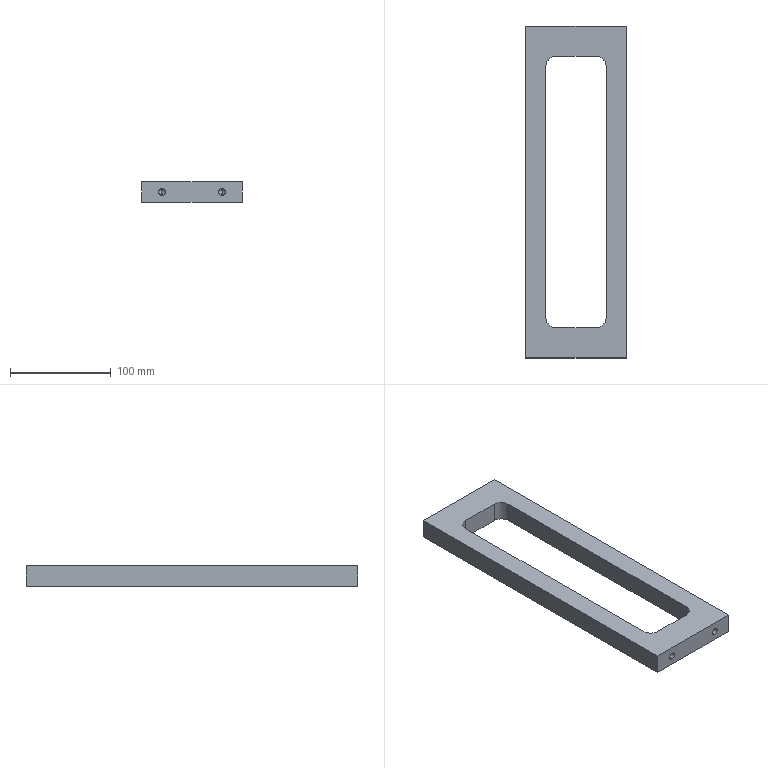Part | SolidWorks | features BaseBody 1 | 1 solid | 22 faces | box 100 x 330 x 20 mm | volume 336233 mm3 | plane 10 | cylinder 8 | cone 4 | commonest cylinder face diameters 6.8 x4 20 x4
STEP:
#1=CARTESIAN_POINT('',(30.,-145.25,3.4));
#2=VERTEX_POINT('',#1);
#3=CARTESIAN_POINT('',(30.,-145.25,-3.4));
#4=VERTEX_POINT('',#3);
#5=CARTESIAN_POINT('',(30.,-145.25,0.));
#6=DIRECTION('',(0.,-1.,0.));
#7=DIRECTION('',(0.,0.,-1.));
#8=AXIS2_PLACEMENT_3D('',#5,#6,#7);
#9=CIRCLE('',#8,3.4);
#10=EDGE_CURVE('',#2,#4,#9,.T.);
#11=ORIENTED_EDGE('',*,*,#10,.F.);
#12=CARTESIAN_POINT('',(30.,-165.,3.4));
#13=VERTEX_POINT('',#12);
#14=CARTESIAN_POINT('',(30.,-165.,3.4));
#15=DIRECTION('',(0.,-1.,0.));
#16=VECTOR('',#15,1000.);
#17=LINE('',#14,#16);
#18=EDGE_CURVE('',#2,#13,#17,.T.);
#19=ORIENTED_EDGE('',*,*,#18,.T.);
#20=CARTESIAN_POINT('',(30.,-165.,-3.4));
#21=VERTEX_POINT('',#20);
#22=CARTESIAN_POINT('',(30.,-165.,0.));
#23=DIRECTION('',(0.,-1.,0.));
#24=DIRECTION('',(0.,0.,-1.));
#25=AXIS2_PLACEMENT_3D('',#22,#23,#24);
#26=CIRCLE('',#25,3.4);
#27=EDGE_CURVE('',#13,#21,#26,.T.);
#28=ORIENTED_EDGE('',*,*,#27,.T.);
#29=CARTESIAN_POINT('',(30.,-165.,-3.4));
#30=DIRECTION('',(0.,-1.,0.));
#31=VECTOR('',#30,1000.);
#32=LINE('',#29,#31);
#33=EDGE_CURVE('',#4,#21,#32,.T.);
#34=ORIENTED_EDGE('',*,*,#33,.F.);
#35=EDGE_LOOP('',(#11,#19,#28,#34));
#36=FACE_OUTER_BOUND('',#35,.T.);
#37=CARTESIAN_POINT('',(30.,-165.,0.));
#38=DIRECTION('',(0.,-1.,0.));
#39=DIRECTION('',(0.,0.,-1.));
#40=AXIS2_PLACEMENT_3D('',#37,#38,#39);
#41=CYLINDRICAL_SURFACE('',#40,3.4);
#42=ADVANCED_FACE('',(#36),#41,.F.);
#43=CARTESIAN_POINT('',(30.,-143.207,0.));
#44=VERTEX_POINT('',#43);
#45=CARTESIAN_POINT('',(30.,-145.25,-3.4));
#46=DIRECTION('',(0.,-0.515,-0.8572));
#47=VECTOR('',#46,1000.);
#48=LINE('',#45,#47);
#49=EDGE_CURVE('',#44,#4,#48,.T.);
#50=ORIENTED_EDGE('',*,*,#49,.F.);
#51=CARTESIAN_POINT('',(30.,-145.25,3.4));
#52=DIRECTION('',(0.,-0.515,0.8572));
#53=VECTOR('',#52,1000.);
#54=LINE('',#51,#53);
#55=EDGE_CURVE('',#44,#2,#54,.T.);
#56=ORIENTED_EDGE('',*,*,#55,.T.);
#57=ORIENTED_EDGE('',*,*,#10,.T.);
#58=EDGE_LOOP('',(#50,#56,#57));
#59=FACE_OUTER_BOUND('',#58,.T.);
#60=CARTESIAN_POINT('',(30.,-145.25,0.));
#61=DIRECTION('',(0.,-1.,0.));
#62=DIRECTION('',(0.,0.,-1.));
#63=AXIS2_PLACEMENT_3D('',#60,#61,#62);
#64=CONICAL_SURFACE('',#63,3.4,1.03);
#65=ADVANCED_FACE('',(#59),#64,.F.);
#66=CARTESIAN_POINT('',(-30.,-145.25,3.4));
#67=VERTEX_POINT('',#66);
#68=CARTESIAN_POINT('',(-30.,-145.25,-3.4));
#69=VERTEX_POINT('',#68);
#70=CARTESIAN_POINT('',(-30.,-145.25,0.));
#71=DIRECTION('',(0.,-1.,0.));
#72=DIRECTION('',(0.,0.,-1.));
#73=AXIS2_PLACEMENT_3D('',#70,#71,#72);
#74=CIRCLE('',#73,3.4);
#75=EDGE_CURVE('',#67,#69,#74,.T.);
#76=ORIENTED_EDGE('',*,*,#75,.F.);
#77=CARTESIAN_POINT('',(-30.,-165.,3.4));
#78=VERTEX_POINT('',#77);
#79=CARTESIAN_POINT('',(-30.,-165.,3.4));
#80=DIRECTION('',(0.,-1.,0.));
#81=VECTOR('',#80,1000.);
#82=LINE('',#79,#81);
#83=EDGE_CURVE('',#67,#78,#82,.T.);
#84=ORIENTED_EDGE('',*,*,#83,.T.);
#85=CARTESIAN_POINT('',(-30.,-165.,-3.4));
#86=VERTEX_POINT('',#85);
#87=CARTESIAN_POINT('',(-30.,-165.,0.));
#88=DIRECTION('',(0.,-1.,0.));
#89=DIRECTION('',(0.,0.,-1.));
#90=AXIS2_PLACEMENT_3D('',#87,#88,#89);
#91=CIRCLE('',#90,3.4);
#92=EDGE_CURVE('',#78,#86,#91,.T.);
#93=ORIENTED_EDGE('',*,*,#92,.T.);
#94=CARTESIAN_POINT('',(-30.,-165.,-3.4));
#95=DIRECTION('',(0.,-1.,0.));
#96=VECTOR('',#95,1000.);
#97=LINE('',#94,#96);
#98=EDGE_CURVE('',#69,#86,#97,.T.);
#99=ORIENTED_EDGE('',*,*,#98,.F.);
#100=EDGE_LOOP('',(#76,#84,#93,#99));
#101=FACE_OUTER_BOUND('',#100,.T.);
#102=CARTESIAN_POINT('',(-30.,-165.,0.));
#103=DIRECTION('',(0.,-1.,0.));
#104=DIRECTION('',(0.,0.,-1.));
#105=AXIS2_PLACEMENT_3D('',#102,#103,#104);
#106=CYLINDRICAL_SURFACE('',#105,3.4);
#107=ADVANCED_FACE('',(#101),#106,.F.);
#108=CARTESIAN_POINT('',(-30.,-143.207,0.));
#109=VERTEX_POINT('',#108);
#110=CARTESIAN_POINT('',(-30.,-145.25,-3.4));
#111=DIRECTION('',(0.,-0.515,-0.8572));
#112=VECTOR('',#111,1000.);
#113=LINE('',#110,#112);
#114=EDGE_CURVE('',#109,#69,#113,.T.);
#115=ORIENTED_EDGE('',*,*,#114,.F.);
#116=CARTESIAN_POINT('',(-30.,-145.25,3.4));
#117=DIRECTION('',(0.,-0.515,0.8572));
#118=VECTOR('',#117,1000.);
#119=LINE('',#116,#118);
#120=EDGE_CURVE('',#109,#67,#119,.T.);
#121=ORIENTED_EDGE('',*,*,#120,.T.);
#122=ORIENTED_EDGE('',*,*,#75,.T.);
#123=EDGE_LOOP('',(#115,#121,#122));
#124=FACE_OUTER_BOUND('',#123,.T.);
#125=CARTESIAN_POINT('',(-30.,-145.25,0.));
#126=DIRECTION('',(0.,-1.,0.));
#127=DIRECTION('',(0.,0.,-1.));
#128=AXIS2_PLACEMENT_3D('',#125,#126,#127);
#129=CONICAL_SURFACE('',#128,3.4,1.03);
#130=ADVANCED_FACE('',(#124),#129,.F.);
#131=CARTESIAN_POINT('',(-50.,165.,-10.));
#132=VERTEX_POINT('',#131);
#133=CARTESIAN_POINT('',(-50.,-165.,-10.));
#134=VERTEX_POINT('',#133);
#135=CARTESIAN_POINT('',(-50.,165.,-10.));
#136=DIRECTION('',(0.,-1.,0.));
#137=VECTOR('',#136,1000.);
#138=LINE('',#135,#137);
#139=EDGE_CURVE('',#132,#134,#138,.T.);
#140=ORIENTED_EDGE('',*,*,#139,.T.);
#141=CARTESIAN_POINT('',(-50.,-165.,10.));
#142=VERTEX_POINT('',#141);
#143=CARTESIAN_POINT('',(-50.,-165.,10.));
#144=DIRECTION('',(0.,0.,-1.));
#145=VECTOR('',#144,1000.);
#146=LINE('',#143,#145);
#147=EDGE_CURVE('',#142,#134,#146,.T.);
#148=ORIENTED_EDGE('',*,*,#147,.F.);
#149=CARTESIAN_POINT('',(-50.,165.,10.));
#150=VERTEX_POINT('',#149);
#151=CARTESIAN_POINT('',(-50.,165.,10.));
#152=DIRECTION('',(0.,-1.,0.));
#153=VECTOR('',#152,1000.);
#154=LINE('',#151,#153);
#155=EDGE_CURVE('',#150,#142,#154,.T.);
#156=ORIENTED_EDGE('',*,*,#155,.F.);
#157=CARTESIAN_POINT('',(-50.,165.,10.));
#158=DIRECTION('',(0.,0.,-1.));
#159=VECTOR('',#158,1000.);
#160=LINE('',#157,#159);
#161=EDGE_CURVE('',#150,#132,#160,.T.);
#162=ORIENTED_EDGE('',*,*,#161,.T.);
#163=EDGE_LOOP('',(#140,#148,#156,#162));
#164=FACE_OUTER_BOUND('',#163,.T.);
#165=CARTESIAN_POINT('',(-50.,165.,10.));
#166=DIRECTION('',(1.,0.,0.));
#167=DIRECTION('',(0.,1.,0.));
#168=AXIS2_PLACEMENT_3D('',#165,#166,#167);
#169=PLANE('',#168);
#170=ADVANCED_FACE('',(#164),#169,.F.);
#171=CARTESIAN_POINT('',(30.,-165.,0.));
#172=DIRECTION('',(0.,-1.,0.));
#173=DIRECTION('',(0.,0.,-1.));
#174=AXIS2_PLACEMENT_3D('',#171,#172,#173);
#175=CIRCLE('',#174,3.4);
#176=EDGE_CURVE('',#21,#13,#175,.T.);
#177=ORIENTED_EDGE('',*,*,#176,.F.);
#178=ORIENTED_EDGE('',*,*,#27,.F.);
#179=EDGE_LOOP('',(#177,#178));
#180=FACE_BOUND('',#179,.T.);
#181=CARTESIAN_POINT('',(-30.,-165.,0.));
#182=DIRECTION('',(0.,-1.,0.));
#183=DIRECTION('',(0.,0.,-1.));
#184=AXIS2_PLACEMENT_3D('',#181,#182,#183);
#185=CIRCLE('',#184,3.4);
#186=EDGE_CURVE('',#86,#78,#185,.T.);
#187=ORIENTED_EDGE('',*,*,#186,.F.);
#188=ORIENTED_EDGE('',*,*,#92,.F.);
#189=EDGE_LOOP('',(#187,#188));
#190=FACE_BOUND('',#189,.T.);
#191=CARTESIAN_POINT('',(50.,-165.,-10.));
#192=VERTEX_POINT('',#191);
#193=CARTESIAN_POINT('',(50.,-165.,-10.));
#194=DIRECTION('',(1.,0.,0.));
#195=VECTOR('',#194,1000.);
#196=LINE('',#193,#195);
#197=EDGE_CURVE('',#134,#192,#196,.T.);
#198=ORIENTED_EDGE('',*,*,#197,.T.);
#199=CARTESIAN_POINT('',(50.,-165.,10.));
#200=VERTEX_POINT('',#199);
#201=CARTESIAN_POINT('',(50.,-165.,10.));
#202=DIRECTION('',(0.,0.,-1.));
#203=VECTOR('',#202,1000.);
#204=LINE('',#201,#203);
#205=EDGE_CURVE('',#200,#192,#204,.T.);
#206=ORIENTED_EDGE('',*,*,#205,.F.);
#207=CARTESIAN_POINT('',(50.,-165.,10.));
#208=DIRECTION('',(1.,0.,0.));
#209=VECTOR('',#208,1000.);
#210=LINE('',#207,#209);
#211=EDGE_CURVE('',#142,#200,#210,.T.);
#212=ORIENTED_EDGE('',*,*,#211,.F.);
#213=ORIENTED_EDGE('',*,*,#147,.T.);
#214=EDGE_LOOP('',(#198,#206,#212,#213));
#215=FACE_OUTER_BOUND('',#214,.T.);
#216=CARTESIAN_POINT('',(50.,-165.,10.));
#217=DIRECTION('',(0.,1.,0.));
#218=DIRECTION('',(0.,0.,1.));
#219=AXIS2_PLACEMENT_3D('',#216,#217,#218);
#220=PLANE('',#219);
#221=ADVANCED_FACE('',(#180,#190,#215),#220,.F.);
#222=CARTESIAN_POINT('',(50.,165.,-10.));
#223=VERTEX_POINT('',#222);
#224=CARTESIAN_POINT('',(50.,165.,-10.));
#225=DIRECTION('',(0.,1.,0.));
#226=VECTOR('',#225,1000.);
#227=LINE('',#224,#226);
#228=EDGE_CURVE('',#192,#223,#227,.T.);
#229=ORIENTED_EDGE('',*,*,#228,.T.);
#230=CARTESIAN_POINT('',(50.,165.,10.));
#231=VERTEX_POINT('',#230);
#232=CARTESIAN_POINT('',(50.,165.,10.));
#233=DIRECTION('',(0.,0.,-1.));
#234=VECTOR('',#233,1000.);
#235=LINE('',#232,#234);
#236=EDGE_CURVE('',#231,#223,#235,.T.);
#237=ORIENTED_EDGE('',*,*,#236,.F.);
#238=CARTESIAN_POINT('',(50.,165.,10.));
#239=DIRECTION('',(0.,1.,0.));
#240=VECTOR('',#239,1000.);
#241=LINE('',#238,#240);
#242=EDGE_CURVE('',#200,#231,#241,.T.);
#243=ORIENTED_EDGE('',*,*,#242,.F.);
#244=ORIENTED_EDGE('',*,*,#205,.T.);
#245=EDGE_LOOP('',(#229,#237,#243,#244));
#246=FACE_OUTER_BOUND('',#245,.T.);
#247=CARTESIAN_POINT('',(50.,165.,10.));
#248=DIRECTION('',(-1.,0.,0.));
#249=DIRECTION('',(0.,-1.,0.));
#250=AXIS2_PLACEMENT_3D('',#247,#248,#249);
#251=PLANE('',#250);
#252=ADVANCED_FACE('',(#246),#251,.F.);
#253=CARTESIAN_POINT('',(50.,165.,-10.));
#254=DIRECTION('',(-1.,0.,0.));
#255=VECTOR('',#254,1000.);
#256=LINE('',#253,#255);
#257=EDGE_CURVE('',#223,#132,#256,.T.);
#258=ORIENTED_EDGE('',*,*,#257,.T.);
#259=ORIENTED_EDGE('',*,*,#161,.F.);
#260=CARTESIAN_POINT('',(50.,165.,10.));
#261=DIRECTION('',(-1.,0.,0.));
#262=VECTOR('',#261,1000.);
#263=LINE('',#260,#262);
#264=EDGE_CURVE('',#231,#150,#263,.T.);
#265=ORIENTED_EDGE('',*,*,#264,.F.);
#266=ORIENTED_EDGE('',*,*,#236,.T.);
#267=EDGE_LOOP('',(#258,#259,#265,#266));
#268=FACE_OUTER_BOUND('',#267,.T.);
#269=CARTESIAN_POINT('',(50.,165.,10.));
#270=DIRECTION('',(0.,-1.,0.));
#271=DIRECTION('',(0.,0.,-1.));
#272=AXIS2_PLACEMENT_3D('',#269,#270,#271);
#273=PLANE('',#272);
#274=ADVANCED_FACE('',(#268),#273,.F.);
#275=CARTESIAN_POINT('',(-20.,-135.,10.));
#276=VERTEX_POINT('',#275);
#277=CARTESIAN_POINT('',(20.,-135.,10.));
#278=VERTEX_POINT('',#277);
#279=CARTESIAN_POINT('',(-20.,-135.,10.));
#280=DIRECTION('',(1.,0.,0.));
#281=VECTOR('',#280,1000.);
#282=LINE('',#279,#281);
#283=EDGE_CURVE('',#276,#278,#282,.T.);
#284=ORIENTED_EDGE('',*,*,#283,.F.);
#285=CARTESIAN_POINT('',(-30.,-125.,10.));
#286=VERTEX_POINT('',#285);
#287=CARTESIAN_POINT('',(-20.,-125.,10.));
#288=DIRECTION('',(0.,0.,1.));
#289=DIRECTION('',(1.,0.,0.));
#290=AXIS2_PLACEMENT_3D('',#287,#288,#289);
#291=CIRCLE('',#290,10.);
#292=EDGE_CURVE('',#286,#276,#291,.T.);
#293=ORIENTED_EDGE('',*,*,#292,.F.);
#294=CARTESIAN_POINT('',(-30.,125.,10.));
#295=VERTEX_POINT('',#294);
#296=CARTESIAN_POINT('',(-30.,125.,10.));
#297=DIRECTION('',(0.,-1.,0.));
#298=VECTOR('',#297,1000.);
#299=LINE('',#296,#298);
#300=EDGE_CURVE('',#295,#286,#299,.T.);
#301=ORIENTED_EDGE('',*,*,#300,.F.);
#302=CARTESIAN_POINT('',(-20.,135.,10.));
#303=VERTEX_POINT('',#302);
#304=CARTESIAN_POINT('',(-20.,125.,10.));
#305=DIRECTION('',(0.,0.,1.));
#306=DIRECTION('',(-1.,0.,0.));
#307=AXIS2_PLACEMENT_3D('',#304,#305,#306);
#308=CIRCLE('',#307,10.);
#309=EDGE_CURVE('',#303,#295,#308,.T.);
#310=ORIENTED_EDGE('',*,*,#309,.F.);
#311=CARTESIAN_POINT('',(20.,135.,10.));
#312=VERTEX_POINT('',#311);
#313=CARTESIAN_POINT('',(-20.,135.,10.));
#314=DIRECTION('',(-1.,0.,0.));
#315=VECTOR('',#314,1000.);
#316=LINE('',#313,#315);
#317=EDGE_CURVE('',#312,#303,#316,.T.);
#318=ORIENTED_EDGE('',*,*,#317,.F.);
#319=CARTESIAN_POINT('',(30.,125.,10.));
#320=VERTEX_POINT('',#319);
#321=CARTESIAN_POINT('',(20.,125.,10.));
#322=DIRECTION('',(0.,0.,1.));
#323=DIRECTION('',(1.,0.,0.));
#324=AXIS2_PLACEMENT_3D('',#321,#322,#323);
#325=CIRCLE('',#324,10.);
#326=EDGE_CURVE('',#320,#312,#325,.T.);
#327=ORIENTED_EDGE('',*,*,#326,.F.);
#328=CARTESIAN_POINT('',(30.,-125.,10.));
#329=VERTEX_POINT('',#328);
#330=CARTESIAN_POINT('',(30.,125.,10.));
#331=DIRECTION('',(0.,1.,0.));
#332=VECTOR('',#331,1000.);
#333=LINE('',#330,#332);
#334=EDGE_CURVE('',#329,#320,#333,.T.);
#335=ORIENTED_EDGE('',*,*,#334,.F.);
#336=CARTESIAN_POINT('',(20.,-125.,10.));
#337=DIRECTION('',(0.,0.,1.));
#338=DIRECTION('',(-1.,0.,0.));
#339=AXIS2_PLACEMENT_3D('',#336,#337,#338);
#340=CIRCLE('',#339,10.);
#341=EDGE_CURVE('',#278,#329,#340,.T.);
#342=ORIENTED_EDGE('',*,*,#341,.F.);
#343=EDGE_LOOP('',(#284,#293,#301,#310,#318,#327,#335,#342));
#344=FACE_BOUND('',#343,.T.);
#345=ORIENTED_EDGE('',*,*,#155,.T.);
#346=ORIENTED_EDGE('',*,*,#211,.T.);
#347=ORIENTED_EDGE('',*,*,#242,.T.);
#348=ORIENTED_EDGE('',*,*,#264,.T.);
#349=EDGE_LOOP('',(#345,#346,#347,#348));
#350=FACE_OUTER_BOUND('',#349,.T.);
#351=CARTESIAN_POINT('',(-50.,-165.,10.));
#352=DIRECTION('',(0.,0.,-1.));
#353=DIRECTION('',(-1.,0.,0.));
#354=AXIS2_PLACEMENT_3D('',#351,#352,#353);
#355=PLANE('',#354);
#356=ADVANCED_FACE('',(#344,#350),#355,.F.);
#357=CARTESIAN_POINT('',(-30.,-125.,-10.));
#358=VERTEX_POINT('',#357);
#359=CARTESIAN_POINT('',(-20.,-135.,-10.));
#360=VERTEX_POINT('',#359);
#361=CARTESIAN_POINT('',(-20.,-125.,-10.));
#362=DIRECTION('',(0.,0.,1.));
#363=DIRECTION('',(1.,0.,0.));
#364=AXIS2_PLACEMENT_3D('',#361,#362,#363);
#365=CIRCLE('',#364,10.);
#366=EDGE_CURVE('',#358,#360,#365,.T.);
#367=ORIENTED_EDGE('',*,*,#366,.T.);
#368=CARTESIAN_POINT('',(20.,-135.,-10.));
#369=VERTEX_POINT('',#368);
#370=CARTESIAN_POINT('',(-20.,-135.,-10.));
#371=DIRECTION('',(1.,0.,0.));
#372=VECTOR('',#371,1000.);
#373=LINE('',#370,#372);
#374=EDGE_CURVE('',#360,#369,#373,.T.);
#375=ORIENTED_EDGE('',*,*,#374,.T.);
#376=CARTESIAN_POINT('',(30.,-125.,-10.));
#377=VERTEX_POINT('',#376);
#378=CARTESIAN_POINT('',(20.,-125.,-10.));
#379=DIRECTION('',(0.,0.,1.));
#380=DIRECTION('',(-1.,0.,0.));
#381=AXIS2_PLACEMENT_3D('',#378,#379,#380);
#382=CIRCLE('',#381,10.);
#383=EDGE_CURVE('',#369,#377,#382,.T.);
#384=ORIENTED_EDGE('',*,*,#383,.T.);
#385=CARTESIAN_POINT('',(30.,125.,-10.));
#386=VERTEX_POINT('',#385);
#387=CARTESIAN_POINT('',(30.,125.,-10.));
#388=DIRECTION('',(0.,1.,0.));
#389=VECTOR('',#388,1000.);
#390=LINE('',#387,#389);
#391=EDGE_CURVE('',#377,#386,#390,.T.);
#392=ORIENTED_EDGE('',*,*,#391,.T.);
#393=CARTESIAN_POINT('',(20.,135.,-10.));
#394=VERTEX_POINT('',#393);
#395=CARTESIAN_POINT('',(20.,125.,-10.));
#396=DIRECTION('',(0.,0.,1.));
#397=DIRECTION('',(1.,0.,0.));
#398=AXIS2_PLACEMENT_3D('',#395,#396,#397);
#399=CIRCLE('',#398,10.);
#400=EDGE_CURVE('',#386,#394,#399,.T.);
#401=ORIENTED_EDGE('',*,*,#400,.T.);
#402=CARTESIAN_POINT('',(-20.,135.,-10.));
#403=VERTEX_POINT('',#402);
#404=CARTESIAN_POINT('',(-20.,135.,-10.));
#405=DIRECTION('',(-1.,0.,0.));
#406=VECTOR('',#405,1000.);
#407=LINE('',#404,#406);
#408=EDGE_CURVE('',#394,#403,#407,.T.);
#409=ORIENTED_EDGE('',*,*,#408,.T.);
#410=CARTESIAN_POINT('',(-30.,125.,-10.));
#411=VERTEX_POINT('',#410);
#412=CARTESIAN_POINT('',(-20.,125.,-10.));
#413=DIRECTION('',(0.,0.,1.));
#414=DIRECTION('',(-1.,0.,0.));
#415=AXIS2_PLACEMENT_3D('',#412,#413,#414);
#416=CIRCLE('',#415,10.);
#417=EDGE_CURVE('',#403,#411,#416,.T.);
#418=ORIENTED_EDGE('',*,*,#417,.T.);
#419=CARTESIAN_POINT('',(-30.,125.,-10.));
#420=DIRECTION('',(0.,-1.,0.));
#421=VECTOR('',#420,1000.);
#422=LINE('',#419,#421);
#423=EDGE_CURVE('',#411,#358,#422,.T.);
#424=ORIENTED_EDGE('',*,*,#423,.T.);
#425=EDGE_LOOP('',(#367,#375,#384,#392,#401,#409,#418,#424));
#426=FACE_BOUND('',#425,.T.);
#427=ORIENTED_EDGE('',*,*,#139,.F.);
#428=ORIENTED_EDGE('',*,*,#257,.F.);
#429=ORIENTED_EDGE('',*,*,#228,.F.);
#430=ORIENTED_EDGE('',*,*,#197,.F.);
#431=EDGE_LOOP('',(#427,#428,#429,#430));
#432=FACE_OUTER_BOUND('',#431,.T.);
#433=CARTESIAN_POINT('',(-50.,-165.,-10.));
#434=DIRECTION('',(0.,0.,-1.));
#435=DIRECTION('',(-1.,0.,0.));
#436=AXIS2_PLACEMENT_3D('',#433,#434,#435);
#437=PLANE('',#436);
#438=ADVANCED_FACE('',(#426,#432),#437,.T.);
#439=ORIENTED_EDGE('',*,*,#292,.T.);
#440=CARTESIAN_POINT('',(-20.,-135.,-10.));
#441=DIRECTION('',(0.,0.,1.));
#442=VECTOR('',#441,1000.);
#443=LINE('',#440,#442);
#444=EDGE_CURVE('',#360,#276,#443,.T.);
#445=ORIENTED_EDGE('',*,*,#444,.F.);
#446=ORIENTED_EDGE('',*,*,#366,.F.);
#447=CARTESIAN_POINT('',(-30.,-125.,-10.));
#448=DIRECTION('',(0.,0.,1.));
#449=VECTOR('',#448,1000.);
#450=LINE('',#447,#449);
#451=EDGE_CURVE('',#358,#286,#450,.T.);
#452=ORIENTED_EDGE('',*,*,#451,.T.);
#453=EDGE_LOOP('',(#439,#445,#446,#452));
#454=FACE_OUTER_BOUND('',#453,.T.);
#455=CARTESIAN_POINT('',(-20.,-125.,-10.));
#456=DIRECTION('',(0.,0.,1.));
#457=DIRECTION('',(1.,0.,0.));
#458=AXIS2_PLACEMENT_3D('',#455,#456,#457);
#459=CYLINDRICAL_SURFACE('',#458,10.);
#460=ADVANCED_FACE('',(#454),#459,.F.);
#461=ORIENTED_EDGE('',*,*,#300,.T.);
#462=ORIENTED_EDGE('',*,*,#451,.F.);
#463=ORIENTED_EDGE('',*,*,#423,.F.);
#464=CARTESIAN_POINT('',(-30.,125.,-10.));
#465=DIRECTION('',(0.,0.,1.));
#466=VECTOR('',#465,1000.);
#467=LINE('',#464,#466);
#468=EDGE_CURVE('',#411,#295,#467,.T.);
#469=ORIENTED_EDGE('',*,*,#468,.T.);
#470=EDGE_LOOP('',(#461,#462,#463,#469));
#471=FACE_OUTER_BOUND('',#470,.T.);
#472=CARTESIAN_POINT('',(-30.,125.,-10.));
#473=DIRECTION('',(-1.,0.,0.));
#474=DIRECTION('',(0.,-1.,0.));
#475=AXIS2_PLACEMENT_3D('',#472,#473,#474);
#476=PLANE('',#475);
#477=ADVANCED_FACE('',(#471),#476,.F.);
#478=ORIENTED_EDGE('',*,*,#309,.T.);
#479=ORIENTED_EDGE('',*,*,#468,.F.);
#480=ORIENTED_EDGE('',*,*,#417,.F.);
#481=CARTESIAN_POINT('',(-20.,135.,-10.));
#482=DIRECTION('',(0.,0.,1.));
#483=VECTOR('',#482,1000.);
#484=LINE('',#481,#483);
#485=EDGE_CURVE('',#403,#303,#484,.T.);
#486=ORIENTED_EDGE('',*,*,#485,.T.);
#487=EDGE_LOOP('',(#478,#479,#480,#486));
#488=FACE_OUTER_BOUND('',#487,.T.);
#489=CARTESIAN_POINT('',(-20.,125.,-10.));
#490=DIRECTION('',(0.,0.,1.));
#491=DIRECTION('',(1.,0.,0.));
#492=AXIS2_PLACEMENT_3D('',#489,#490,#491);
#493=CYLINDRICAL_SURFACE('',#492,10.);
#494=ADVANCED_FACE('',(#488),#493,.F.);
#495=ORIENTED_EDGE('',*,*,#317,.T.);
#496=ORIENTED_EDGE('',*,*,#485,.F.);
#497=ORIENTED_EDGE('',*,*,#408,.F.);
#498=CARTESIAN_POINT('',(20.,135.,-10.));
#499=DIRECTION('',(0.,0.,1.));
#500=VECTOR('',#499,1000.);
#501=LINE('',#498,#500);
#502=EDGE_CURVE('',#394,#312,#501,.T.);
#503=ORIENTED_EDGE('',*,*,#502,.T.);
#504=EDGE_LOOP('',(#495,#496,#497,#503));
#505=FACE_OUTER_BOUND('',#504,.T.);
#506=CARTESIAN_POINT('',(-20.,135.,-10.));
#507=DIRECTION('',(0.,1.,0.));
#508=DIRECTION('',(0.,0.,1.));
#509=AXIS2_PLACEMENT_3D('',#506,#507,#508);
#510=PLANE('',#509);
#511=ADVANCED_FACE('',(#505),#510,.F.);
#512=ORIENTED_EDGE('',*,*,#326,.T.);
#513=ORIENTED_EDGE('',*,*,#502,.F.);
#514=ORIENTED_EDGE('',*,*,#400,.F.);
#515=CARTESIAN_POINT('',(30.,125.,-10.));
#516=DIRECTION('',(0.,0.,1.));
#517=VECTOR('',#516,1000.);
#518=LINE('',#515,#517);
#519=EDGE_CURVE('',#386,#320,#518,.T.);
#520=ORIENTED_EDGE('',*,*,#519,.T.);
#521=EDGE_LOOP('',(#512,#513,#514,#520));
#522=FACE_OUTER_BOUND('',#521,.T.);
#523=CARTESIAN_POINT('',(20.,125.,-10.));
#524=DIRECTION('',(0.,0.,1.));
#525=DIRECTION('',(1.,0.,0.));
#526=AXIS2_PLACEMENT_3D('',#523,#524,#525);
#527=CYLINDRICAL_SURFACE('',#526,10.);
#528=ADVANCED_FACE('',(#522),#527,.F.);
#529=ORIENTED_EDGE('',*,*,#334,.T.);
#530=ORIENTED_EDGE('',*,*,#519,.F.);
#531=ORIENTED_EDGE('',*,*,#391,.F.);
#532=CARTESIAN_POINT('',(30.,-125.,-10.));
#533=DIRECTION('',(0.,0.,1.));
#534=VECTOR('',#533,1000.);
#535=LINE('',#532,#534);
#536=EDGE_CURVE('',#377,#329,#535,.T.);
#537=ORIENTED_EDGE('',*,*,#536,.T.);
#538=EDGE_LOOP('',(#529,#530,#531,#537));
#539=FACE_OUTER_BOUND('',#538,.T.);
#540=CARTESIAN_POINT('',(30.,125.,-10.));
#541=DIRECTION('',(1.,0.,0.));
#542=DIRECTION('',(0.,1.,0.));
#543=AXIS2_PLACEMENT_3D('',#540,#541,#542);
#544=PLANE('',#543);
#545=ADVANCED_FACE('',(#539),#544,.F.);
#546=ORIENTED_EDGE('',*,*,#341,.T.);
#547=ORIENTED_EDGE('',*,*,#536,.F.);
#548=ORIENTED_EDGE('',*,*,#383,.F.);
#549=CARTESIAN_POINT('',(20.,-135.,-10.));
#550=DIRECTION('',(0.,0.,1.));
#551=VECTOR('',#550,1000.);
#552=LINE('',#549,#551);
#553=EDGE_CURVE('',#369,#278,#552,.T.);
#554=ORIENTED_EDGE('',*,*,#553,.T.);
#555=EDGE_LOOP('',(#546,#547,#548,#554));
#556=FACE_OUTER_BOUND('',#555,.T.);
#557=CARTESIAN_POINT('',(20.,-125.,-10.));
#558=DIRECTION('',(0.,0.,1.));
#559=DIRECTION('',(1.,0.,0.));
#560=AXIS2_PLACEMENT_3D('',#557,#558,#559);
#561=CYLINDRICAL_SURFACE('',#560,10.);
#562=ADVANCED_FACE('',(#556),#561,.F.);
#563=ORIENTED_EDGE('',*,*,#283,.T.);
#564=ORIENTED_EDGE('',*,*,#553,.F.);
#565=ORIENTED_EDGE('',*,*,#374,.F.);
#566=ORIENTED_EDGE('',*,*,#444,.T.);
#567=EDGE_LOOP('',(#563,#564,#565,#566));
#568=FACE_OUTER_BOUND('',#567,.T.);
#569=CARTESIAN_POINT('',(-20.,-135.,-10.));
#570=DIRECTION('',(0.,-1.,0.));
#571=DIRECTION('',(0.,0.,-1.));
#572=AXIS2_PLACEMENT_3D('',#569,#570,#571);
#573=PLANE('',#572);
#574=ADVANCED_FACE('',(#568),#573,.F.);
#575=ORIENTED_EDGE('',*,*,#120,.F.);
#576=ORIENTED_EDGE('',*,*,#114,.T.);
#577=CARTESIAN_POINT('',(-30.,-145.25,0.));
#578=DIRECTION('',(0.,-1.,0.));
#579=DIRECTION('',(0.,0.,-1.));
#580=AXIS2_PLACEMENT_3D('',#577,#578,#579);
#581=CIRCLE('',#580,3.4);
#582=EDGE_CURVE('',#69,#67,#581,.T.);
#583=ORIENTED_EDGE('',*,*,#582,.T.);
#584=EDGE_LOOP('',(#575,#576,#583));
#585=FACE_OUTER_BOUND('',#584,.T.);
#586=CARTESIAN_POINT('',(-30.,-145.25,0.));
#587=DIRECTION('',(0.,-1.,0.));
#588=DIRECTION('',(0.,0.,-1.));
#589=AXIS2_PLACEMENT_3D('',#586,#587,#588);
#590=CONICAL_SURFACE('',#589,3.4,1.03);
#591=ADVANCED_FACE('',(#585),#590,.F.);
#592=ORIENTED_EDGE('',*,*,#83,.F.);
#593=ORIENTED_EDGE('',*,*,#582,.F.);
#594=ORIENTED_EDGE('',*,*,#98,.T.);
#595=ORIENTED_EDGE('',*,*,#186,.T.);
#596=EDGE_LOOP('',(#592,#593,#594,#595));
#597=FACE_OUTER_BOUND('',#596,.T.);
#598=CARTESIAN_POINT('',(-30.,-165.,0.));
#599=DIRECTION('',(0.,-1.,0.));
#600=DIRECTION('',(0.,0.,-1.));
#601=AXIS2_PLACEMENT_3D('',#598,#599,#600);
#602=CYLINDRICAL_SURFACE('',#601,3.4);
#603=ADVANCED_FACE('',(#597),#602,.F.);
#604=ORIENTED_EDGE('',*,*,#55,.F.);
#605=ORIENTED_EDGE('',*,*,#49,.T.);
#606=CARTESIAN_POINT('',(30.,-145.25,0.));
#607=DIRECTION('',(0.,-1.,0.));
#608=DIRECTION('',(0.,0.,-1.));
#609=AXIS2_PLACEMENT_3D('',#606,#607,#608);
#610=CIRCLE('',#609,3.4);
#611=EDGE_CURVE('',#4,#2,#610,.T.);
#612=ORIENTED_EDGE('',*,*,#611,.T.);
#613=EDGE_LOOP('',(#604,#605,#612));
#614=FACE_OUTER_BOUND('',#613,.T.);
#615=CARTESIAN_POINT('',(30.,-145.25,0.));
#616=DIRECTION('',(0.,-1.,0.));
#617=DIRECTION('',(0.,0.,-1.));
#618=AXIS2_PLACEMENT_3D('',#615,#616,#617);
#619=CONICAL_SURFACE('',#618,3.4,1.03);
#620=ADVANCED_FACE('',(#614),#619,.F.);
#621=ORIENTED_EDGE('',*,*,#18,.F.);
#622=ORIENTED_EDGE('',*,*,#611,.F.);
#623=ORIENTED_EDGE('',*,*,#33,.T.);
#624=ORIENTED_EDGE('',*,*,#176,.T.);
#625=EDGE_LOOP('',(#621,#622,#623,#624));
#626=FACE_OUTER_BOUND('',#625,.T.);
#627=CARTESIAN_POINT('',(30.,-165.,0.));
#628=DIRECTION('',(0.,-1.,0.));
#629=DIRECTION('',(0.,0.,-1.));
#630=AXIS2_PLACEMENT_3D('',#627,#628,#629);
#631=CYLINDRICAL_SURFACE('',#630,3.4);
#632=ADVANCED_FACE('',(#626),#631,.F.);
#633=CLOSED_SHELL('',(#42,#65,#107,#130,#170,#221,#252,#274,#356,#438,#460,#477,#494,#511,#528,#545,#562,#574,#591,#603,#620,#632));
#634=MANIFOLD_SOLID_BREP('',#633);
#635=CARTESIAN_POINT('',(0.,0.,0.));
#636=DIRECTION('',(0.,0.,1.));
#637=DIRECTION('',(1.,0.,0.));
#638=AXIS2_PLACEMENT_3D('',#635,#636,#637);
#639=(LENGTH_UNIT()NAMED_UNIT(*)SI_UNIT(.MILLI.,.METRE.));
#640=UNCERTAINTY_MEASURE_WITH_UNIT(LENGTH_MEASURE(0.00001),#639,'','');
#641=(NAMED_UNIT(*)PLANE_ANGLE_UNIT()SI_UNIT($,.RADIAN.));
#642=(NAMED_UNIT(*)SI_UNIT($,.STERADIAN.)SOLID_ANGLE_UNIT());
#643=(GEOMETRIC_REPRESENTATION_CONTEXT(3)GLOBAL_UNCERTAINTY_ASSIGNED_CONTEXT((#640))GLOBAL_UNIT_ASSIGNED_CONTEXT((#639,#641,#642))REPRESENTATION_CONTEXT('',''));
#644=ADVANCED_BREP_SHAPE_REPRESENTATION('',(#634,#638),#643);